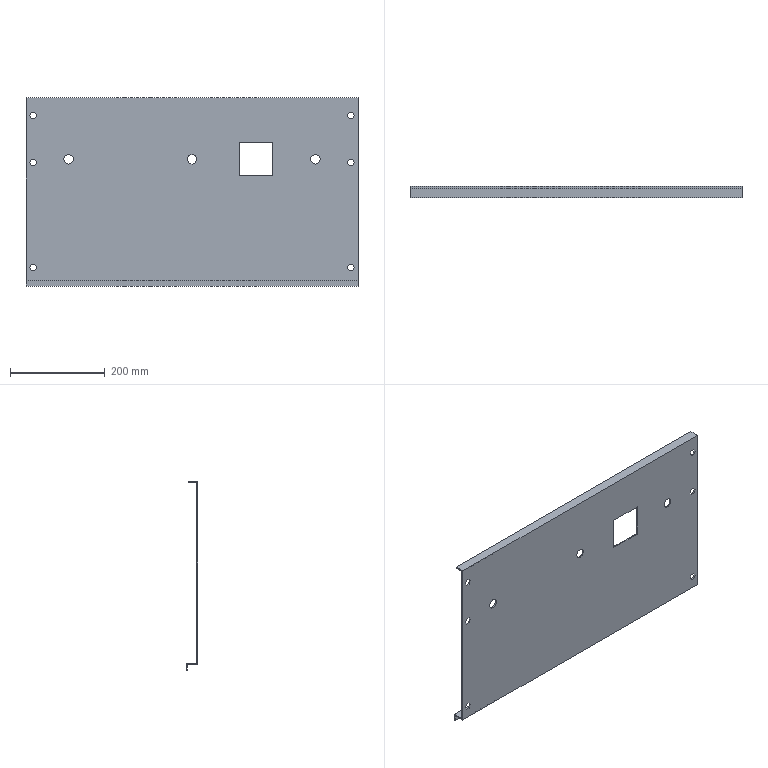Part | SolidWorks | features BaseBody 1 | 1 solid | 58 faces | box 700 x 25 x 397.5 mm | volume 748823 mm3 | plane 52 | cylinder 6 | commonest cylinder face diameters 20 x6